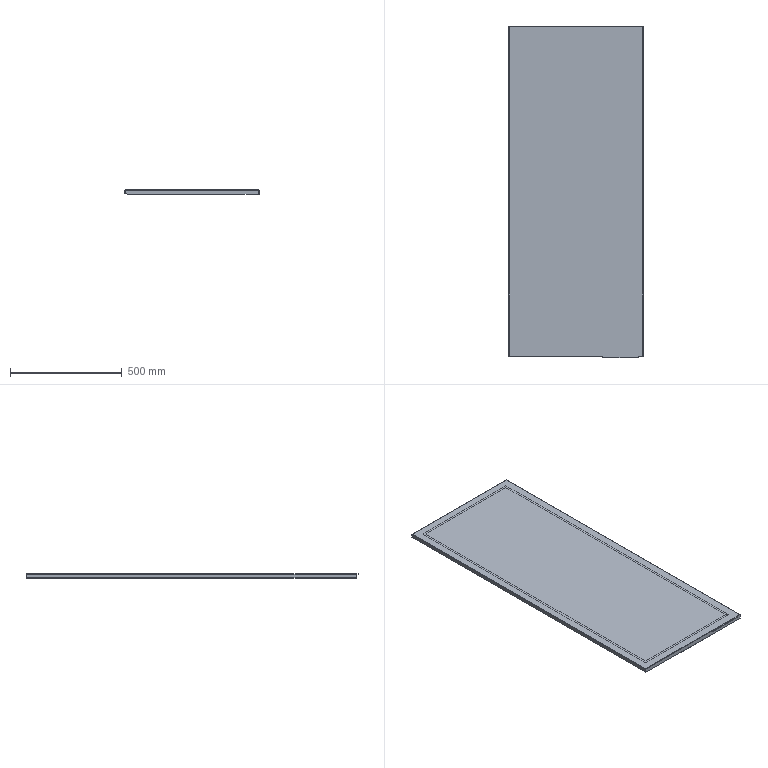Part | SolidWorks | features ICE 6, MoveFace 6, BaseBody 1 | 1 solid | 64 faces | box 599 x 1482 x 20 mm | volume 2481350 mm3 | plane 56 | cylinder 8 | commonest cylinder face diameters 0.2 x4 4.2 x4